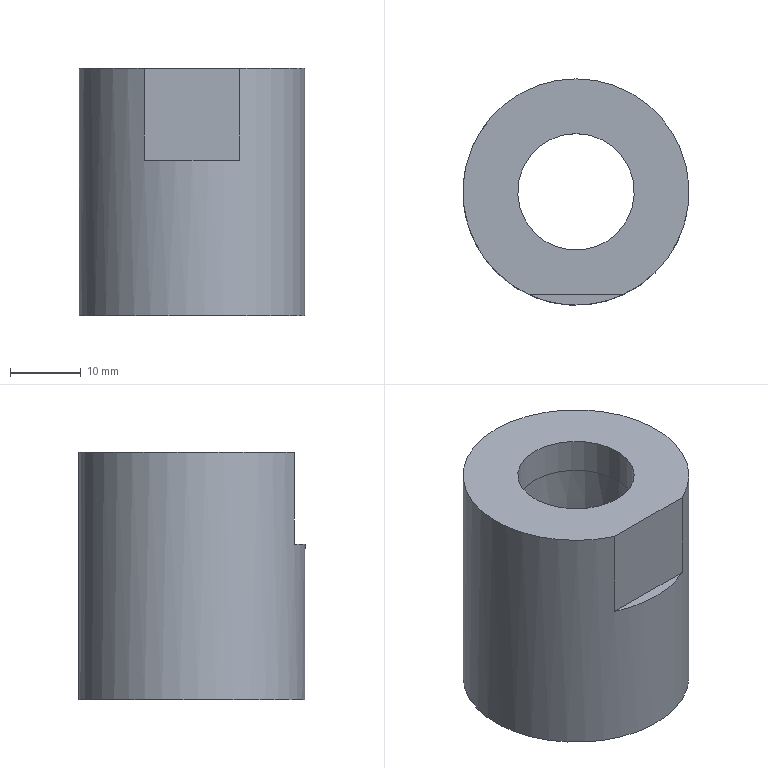Part | STEP file | lll_id4074_x_t | 1 solid | 7 faces | box 32 x 32 x 35 mm | volume 19857 mm3 | plane 4 | cylinder 2 | cone 1 | commonest cylinder face diameters 16.5 x1 32 x1
STEP:
#1=CARTESIAN_POINT('',(443.764,285.5,-13.));
#2=VERTEX_POINT('',#1);
#3=CARTESIAN_POINT('',(430.236,285.5,-13.));
#4=VERTEX_POINT('',#3);
#5=CARTESIAN_POINT('',(437.,285.5,-13.));
#6=DIRECTION('',(-1.,0.,0.));
#7=VECTOR('',#6,1.);
#8=LINE('',#5,#7);
#9=EDGE_CURVE('',#2,#4,#8,.T.);
#10=ORIENTED_EDGE('',*,*,#9,.F.);
#11=CARTESIAN_POINT('',(443.764,285.5,0.));
#12=VERTEX_POINT('',#11);
#13=CARTESIAN_POINT('',(443.764,285.5,-15.));
#14=DIRECTION('',(0.,0.,-1.));
#15=VECTOR('',#14,1.);
#16=LINE('',#13,#15);
#17=EDGE_CURVE('',#12,#2,#16,.T.);
#18=ORIENTED_EDGE('',*,*,#17,.F.);
#19=CARTESIAN_POINT('',(430.236,285.5,0.));
#20=VERTEX_POINT('',#19);
#21=CARTESIAN_POINT('',(437.,285.5,0.));
#22=DIRECTION('',(1.,0.,0.));
#23=VECTOR('',#22,1.);
#24=LINE('',#21,#23);
#25=EDGE_CURVE('',#20,#12,#24,.T.);
#26=ORIENTED_EDGE('',*,*,#25,.F.);
#27=CARTESIAN_POINT('',(430.236,285.5,-15.));
#28=DIRECTION('',(0.,0.,1.));
#29=VECTOR('',#28,1.);
#30=LINE('',#27,#29);
#31=EDGE_CURVE('',#4,#20,#30,.T.);
#32=ORIENTED_EDGE('',*,*,#31,.F.);
#33=EDGE_LOOP('',(#10,#18,#26,#32));
#34=FACE_OUTER_BOUND('',#33,.T.);
#35=CARTESIAN_POINT('',(424.875,285.5,-17.5));
#36=DIRECTION('',(0.,1.,0.));
#37=DIRECTION('',(0.,0.,1.));
#38=AXIS2_PLACEMENT_3D('',#35,#36,#37);
#39=PLANE('',#38);
#40=ADVANCED_FACE('',(#34),#39,.F.);
#41=CARTESIAN_POINT('',(437.,308.25,-5.));
#42=VERTEX_POINT('',#41);
#43=CARTESIAN_POINT('',(437.,300.,-5.));
#44=DIRECTION('',(0.,0.,1.));
#45=DIRECTION('',(0.,1.,0.));
#46=AXIS2_PLACEMENT_3D('',#43,#44,#45);
#47=CIRCLE('',#46,8.25);
#48=EDGE_CURVE('',#42,#42,#47,.T.);
#49=ORIENTED_EDGE('',*,*,#48,.T.);
#50=EDGE_LOOP('',(#49));
#51=FACE_BOUND('',#50,.T.);
#52=CARTESIAN_POINT('',(437.,290.964,-35.));
#53=VERTEX_POINT('',#52);
#54=CARTESIAN_POINT('',(437.,300.,-35.));
#55=DIRECTION('',(0.,0.,1.));
#56=DIRECTION('',(0.,-1.,0.));
#57=AXIS2_PLACEMENT_3D('',#54,#55,#56);
#58=CIRCLE('',#57,9.036);
#59=EDGE_CURVE('',#53,#53,#58,.T.);
#60=ORIENTED_EDGE('',*,*,#59,.F.);
#61=EDGE_LOOP('',(#60));
#62=FACE_BOUND('',#61,.T.);
#63=CARTESIAN_POINT('',(437.,300.,-5.));
#64=DIRECTION('',(0.,0.,-1.));
#65=DIRECTION('',(0.,1.,0.));
#66=AXIS2_PLACEMENT_3D('',#63,#64,#65);
#67=CONICAL_SURFACE('',#66,8.25,1.5);
#68=ADVANCED_FACE('',(#51,#62),#67,.F.);
#69=CARTESIAN_POINT('',(437.,308.25,0.));
#70=VERTEX_POINT('',#69);
#71=CARTESIAN_POINT('',(437.,300.,0.));
#72=DIRECTION('',(0.,0.,1.));
#73=DIRECTION('',(0.,1.,0.));
#74=AXIS2_PLACEMENT_3D('',#71,#72,#73);
#75=CIRCLE('',#74,8.25);
#76=EDGE_CURVE('',#70,#70,#75,.T.);
#77=ORIENTED_EDGE('',*,*,#76,.T.);
#78=EDGE_LOOP('',(#77));
#79=FACE_BOUND('',#78,.T.);
#80=ORIENTED_EDGE('',*,*,#48,.F.);
#81=EDGE_LOOP('',(#80));
#82=FACE_BOUND('',#81,.T.);
#83=CARTESIAN_POINT('',(437.,300.,-2.4));
#84=DIRECTION('',(0.,0.,1.));
#85=DIRECTION('',(0.,1.,0.));
#86=AXIS2_PLACEMENT_3D('',#83,#84,#85);
#87=CYLINDRICAL_SURFACE('',#86,8.25);
#88=ADVANCED_FACE('',(#79,#82),#87,.F.);
#89=ORIENTED_EDGE('',*,*,#76,.F.);
#90=EDGE_LOOP('',(#89));
#91=FACE_BOUND('',#90,.T.);
#92=CARTESIAN_POINT('',(437.,300.,0.));
#93=DIRECTION('',(0.,0.,1.));
#94=DIRECTION('',(0.,1.,0.));
#95=AXIS2_PLACEMENT_3D('',#92,#93,#94);
#96=CIRCLE('',#95,16.);
#97=EDGE_CURVE('',#12,#20,#96,.T.);
#98=ORIENTED_EDGE('',*,*,#97,.T.);
#99=ORIENTED_EDGE('',*,*,#25,.T.);
#100=EDGE_LOOP('',(#98,#99));
#101=FACE_BOUND('',#100,.T.);
#102=CARTESIAN_POINT('',(437.,300.,0.));
#103=DIRECTION('',(0.,0.,1.));
#104=DIRECTION('',(0.,-1.,0.));
#105=AXIS2_PLACEMENT_3D('',#102,#103,#104);
#106=PLANE('',#105);
#107=ADVANCED_FACE('',(#91,#101),#106,.T.);
#108=ORIENTED_EDGE('',*,*,#17,.T.);
#109=CARTESIAN_POINT('',(437.,300.,-13.));
#110=DIRECTION('',(0.,0.,1.));
#111=DIRECTION('',(1.,0.,0.));
#112=AXIS2_PLACEMENT_3D('',#109,#110,#111);
#113=CIRCLE('',#112,16.);
#114=EDGE_CURVE('',#4,#2,#113,.T.);
#115=ORIENTED_EDGE('',*,*,#114,.F.);
#116=ORIENTED_EDGE('',*,*,#31,.T.);
#117=ORIENTED_EDGE('',*,*,#97,.F.);
#118=EDGE_LOOP('',(#108,#115,#116,#117));
#119=FACE_BOUND('',#118,.T.);
#120=CARTESIAN_POINT('',(437.,316.,-35.));
#121=VERTEX_POINT('',#120);
#122=CARTESIAN_POINT('',(437.,300.,-35.));
#123=DIRECTION('',(0.,0.,-1.));
#124=DIRECTION('',(0.,1.,0.));
#125=AXIS2_PLACEMENT_3D('',#122,#123,#124);
#126=CIRCLE('',#125,16.);
#127=EDGE_CURVE('',#121,#121,#126,.T.);
#128=ORIENTED_EDGE('',*,*,#127,.F.);
#129=EDGE_LOOP('',(#128));
#130=FACE_BOUND('',#129,.T.);
#131=CARTESIAN_POINT('',(437.,300.,-15.));
#132=DIRECTION('',(0.,0.,-1.));
#133=DIRECTION('',(1.,0.,0.));
#134=AXIS2_PLACEMENT_3D('',#131,#132,#133);
#135=CYLINDRICAL_SURFACE('',#134,16.);
#136=ADVANCED_FACE('',(#119,#130),#135,.T.);
#137=ORIENTED_EDGE('',*,*,#127,.T.);
#138=EDGE_LOOP('',(#137));
#139=FACE_BOUND('',#138,.T.);
#140=ORIENTED_EDGE('',*,*,#59,.T.);
#141=EDGE_LOOP('',(#140));
#142=FACE_BOUND('',#141,.T.);
#143=CARTESIAN_POINT('',(442.5,300.,-35.));
#144=DIRECTION('',(0.,0.,-1.));
#145=DIRECTION('',(-1.,0.,0.));
#146=AXIS2_PLACEMENT_3D('',#143,#144,#145);
#147=PLANE('',#146);
#148=ADVANCED_FACE('',(#139,#142),#147,.T.);
#149=ORIENTED_EDGE('',*,*,#114,.T.);
#150=ORIENTED_EDGE('',*,*,#9,.T.);
#151=EDGE_LOOP('',(#149,#150));
#152=FACE_OUTER_BOUND('',#151,.T.);
#153=CARTESIAN_POINT('',(437.,300.,-13.));
#154=DIRECTION('',(0.,0.,1.));
#155=DIRECTION('',(0.,-1.,0.));
#156=AXIS2_PLACEMENT_3D('',#153,#154,#155);
#157=PLANE('',#156);
#158=ADVANCED_FACE('',(#152),#157,.T.);
#159=CLOSED_SHELL('',(#40,#68,#88,#107,#136,#148,#158));
#160=MANIFOLD_SOLID_BREP('',#159);
#161=(LENGTH_UNIT()NAMED_UNIT(*)SI_UNIT(.MILLI.,.METRE.));
#162=UNCERTAINTY_MEASURE_WITH_UNIT(LENGTH_MEASURE(0.00002),#161,'','');
#163=(NAMED_UNIT(*)PLANE_ANGLE_UNIT()SI_UNIT($,.RADIAN.));
#164=PLANE_ANGLE_MEASURE_WITH_UNIT(PLANE_ANGLE_MEASURE(0.01745),#163);
#165=DIMENSIONAL_EXPONENTS(0.,0.,0.,0.,0.,0.,0.);
#166=(CONVERSION_BASED_UNIT('DEGREE',#164)NAMED_UNIT(#165)PLANE_ANGLE_UNIT());
#167=(NAMED_UNIT(*)SI_UNIT($,.STERADIAN.)SOLID_ANGLE_UNIT());
#168=(GEOMETRIC_REPRESENTATION_CONTEXT(3)GLOBAL_UNCERTAINTY_ASSIGNED_CONTEXT((#162))GLOBAL_UNIT_ASSIGNED_CONTEXT((#161,#166,#167))REPRESENTATION_CONTEXT('',''));
#169=ADVANCED_BREP_SHAPE_REPRESENTATION('',(#160),#168);